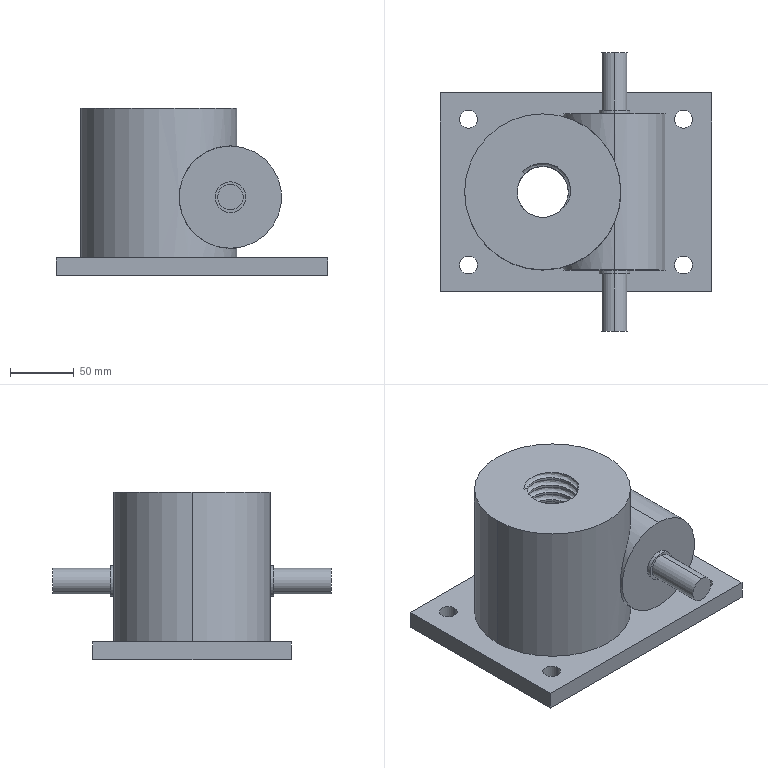Part | SolidWorks | features ICE 6, Extrusion 1, Helix 1, MirrorSolid 1, RefAxis 1, SweepCut 1 | 5 solids | 72 faces | volume 2041758 mm3 | cylinder 52 | plane 19 | spline 1 | commonest cylinder face diameters 40 x31 14 x8 20 x4 24 x4 80 x3 122 x2